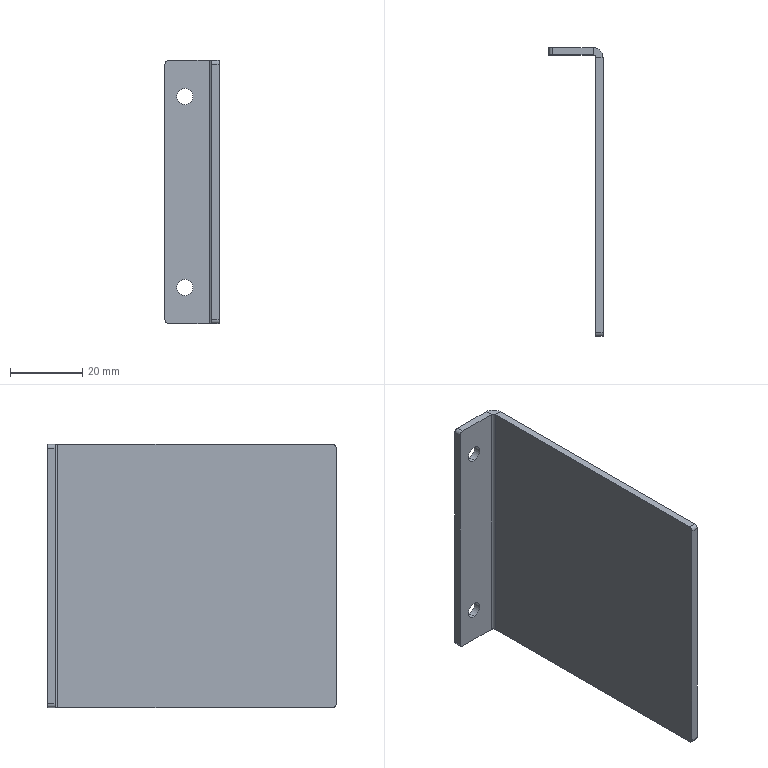Part | STEP file | 11-FG-B07311 | 1 solid | 22 faces | box 15 x 80 x 73 mm | volume 13404 mm3 | plane 12 | cylinder 10 | commonest cylinder face diameters 2 x4 4.5 x4 1.473 x1 5.473 x1
STEP:
#1=CARTESIAN_POINT('',(5.5,-2.,7.75));
#2=VERTEX_POINT('',#1);
#3=CARTESIAN_POINT('',(5.5,-2.,12.25));
#4=VERTEX_POINT('',#3);
#5=CARTESIAN_POINT('',(5.5,-2.,10.));
#6=DIRECTION('',(0.,1.,0.));
#7=DIRECTION('',(0.,0.,1.));
#8=AXIS2_PLACEMENT_3D('',#5,#6,#7);
#9=CIRCLE('',#8,2.25);
#10=EDGE_CURVE('',#2,#4,#9,.T.);
#11=ORIENTED_EDGE('',*,*,#10,.F.);
#12=CARTESIAN_POINT('',(5.5,0.,7.75));
#13=VERTEX_POINT('',#12);
#14=CARTESIAN_POINT('',(5.5,-10.,7.75));
#15=DIRECTION('',(0.,1.,0.));
#16=VECTOR('',#15,1000.);
#17=LINE('',#14,#16);
#18=EDGE_CURVE('',#2,#13,#17,.T.);
#19=ORIENTED_EDGE('',*,*,#18,.T.);
#20=CARTESIAN_POINT('',(5.5,0.,12.25));
#21=VERTEX_POINT('',#20);
#22=CARTESIAN_POINT('',(5.5,0.,10.));
#23=DIRECTION('',(0.,1.,0.));
#24=DIRECTION('',(0.,0.,1.));
#25=AXIS2_PLACEMENT_3D('',#22,#23,#24);
#26=CIRCLE('',#25,2.25);
#27=EDGE_CURVE('',#13,#21,#26,.T.);
#28=ORIENTED_EDGE('',*,*,#27,.T.);
#29=CARTESIAN_POINT('',(5.5,-10.,12.25));
#30=DIRECTION('',(0.,1.,0.));
#31=VECTOR('',#30,1000.);
#32=LINE('',#29,#31);
#33=EDGE_CURVE('',#4,#21,#32,.T.);
#34=ORIENTED_EDGE('',*,*,#33,.F.);
#35=EDGE_LOOP('',(#11,#19,#28,#34));
#36=FACE_OUTER_BOUND('',#35,.T.);
#37=CARTESIAN_POINT('',(5.5,-10.,10.));
#38=DIRECTION('',(0.,1.,0.));
#39=DIRECTION('',(0.,0.,1.));
#40=AXIS2_PLACEMENT_3D('',#37,#38,#39);
#41=CYLINDRICAL_SURFACE('',#40,2.25);
#42=ADVANCED_FACE('',(#36),#41,.F.);
#43=CARTESIAN_POINT('',(5.5,-2.,60.75));
#44=VERTEX_POINT('',#43);
#45=CARTESIAN_POINT('',(5.5,-2.,65.25));
#46=VERTEX_POINT('',#45);
#47=CARTESIAN_POINT('',(5.5,-2.,63.));
#48=DIRECTION('',(0.,1.,0.));
#49=DIRECTION('',(0.,0.,1.));
#50=AXIS2_PLACEMENT_3D('',#47,#48,#49);
#51=CIRCLE('',#50,2.25);
#52=EDGE_CURVE('',#44,#46,#51,.T.);
#53=ORIENTED_EDGE('',*,*,#52,.F.);
#54=CARTESIAN_POINT('',(5.5,0.,60.75));
#55=VERTEX_POINT('',#54);
#56=CARTESIAN_POINT('',(5.5,-10.,60.75));
#57=DIRECTION('',(0.,1.,0.));
#58=VECTOR('',#57,1000.);
#59=LINE('',#56,#58);
#60=EDGE_CURVE('',#44,#55,#59,.T.);
#61=ORIENTED_EDGE('',*,*,#60,.T.);
#62=CARTESIAN_POINT('',(5.5,0.,65.25));
#63=VERTEX_POINT('',#62);
#64=CARTESIAN_POINT('',(5.5,0.,63.));
#65=DIRECTION('',(0.,1.,0.));
#66=DIRECTION('',(0.,0.,1.));
#67=AXIS2_PLACEMENT_3D('',#64,#65,#66);
#68=CIRCLE('',#67,2.25);
#69=EDGE_CURVE('',#55,#63,#68,.T.);
#70=ORIENTED_EDGE('',*,*,#69,.T.);
#71=CARTESIAN_POINT('',(5.5,-10.,65.25));
#72=DIRECTION('',(0.,1.,0.));
#73=VECTOR('',#72,1000.);
#74=LINE('',#71,#73);
#75=EDGE_CURVE('',#46,#63,#74,.T.);
#76=ORIENTED_EDGE('',*,*,#75,.F.);
#77=EDGE_LOOP('',(#53,#61,#70,#76));
#78=FACE_OUTER_BOUND('',#77,.T.);
#79=CARTESIAN_POINT('',(5.5,-10.,63.));
#80=DIRECTION('',(0.,1.,0.));
#81=DIRECTION('',(0.,0.,1.));
#82=AXIS2_PLACEMENT_3D('',#79,#80,#81);
#83=CYLINDRICAL_SURFACE('',#82,2.25);
#84=ADVANCED_FACE('',(#78),#83,.F.);
#85=CARTESIAN_POINT('',(15.,-2.737,73.));
#86=VERTEX_POINT('',#85);
#87=CARTESIAN_POINT('',(13.,-2.737,73.));
#88=VERTEX_POINT('',#87);
#89=CARTESIAN_POINT('',(15.,-2.737,73.));
#90=DIRECTION('',(-1.,0.,0.));
#91=VECTOR('',#90,1000.);
#92=LINE('',#89,#91);
#93=EDGE_CURVE('',#86,#88,#92,.T.);
#94=ORIENTED_EDGE('',*,*,#93,.F.);
#95=CARTESIAN_POINT('',(12.263,0.,73.));
#96=VERTEX_POINT('',#95);
#97=CARTESIAN_POINT('',(12.263,-2.737,73.));
#98=DIRECTION('',(0.,0.,-1.));
#99=DIRECTION('',(1.,0.,0.));
#100=AXIS2_PLACEMENT_3D('',#97,#98,#99);
#101=CIRCLE('',#100,2.737);
#102=EDGE_CURVE('',#96,#86,#101,.T.);
#103=ORIENTED_EDGE('',*,*,#102,.F.);
#104=CARTESIAN_POINT('',(12.263,-2.,73.));
#105=VERTEX_POINT('',#104);
#106=CARTESIAN_POINT('',(12.263,-2.,73.));
#107=DIRECTION('',(0.,1.,0.));
#108=VECTOR('',#107,1000.);
#109=LINE('',#106,#108);
#110=EDGE_CURVE('',#105,#96,#109,.T.);
#111=ORIENTED_EDGE('',*,*,#110,.F.);
#112=CARTESIAN_POINT('',(12.263,-2.737,73.));
#113=DIRECTION('',(0.,0.,-1.));
#114=DIRECTION('',(1.,0.,0.));
#115=AXIS2_PLACEMENT_3D('',#112,#113,#114);
#116=CIRCLE('',#115,0.7366);
#117=EDGE_CURVE('',#105,#88,#116,.T.);
#118=ORIENTED_EDGE('',*,*,#117,.T.);
#119=EDGE_LOOP('',(#94,#103,#111,#118));
#120=FACE_OUTER_BOUND('',#119,.T.);
#121=CARTESIAN_POINT('',(15.,-2.737,73.));
#122=DIRECTION('',(0.,0.,1.));
#123=DIRECTION('',(1.,0.,0.));
#124=AXIS2_PLACEMENT_3D('',#121,#122,#123);
#125=PLANE('',#124);
#126=ADVANCED_FACE('',(#120),#125,.T.);
#127=CARTESIAN_POINT('',(13.,-79.,73.));
#128=VERTEX_POINT('',#127);
#129=CARTESIAN_POINT('',(13.,0.,73.));
#130=DIRECTION('',(0.,-1.,0.));
#131=VECTOR('',#130,1000.);
#132=LINE('',#129,#131);
#133=EDGE_CURVE('',#88,#128,#132,.T.);
#134=ORIENTED_EDGE('',*,*,#133,.T.);
#135=CARTESIAN_POINT('',(15.,-79.,73.));
#136=VERTEX_POINT('',#135);
#137=CARTESIAN_POINT('',(12.263,-79.,73.));
#138=DIRECTION('',(1.,0.,0.));
#139=VECTOR('',#138,1000.);
#140=LINE('',#137,#139);
#141=EDGE_CURVE('',#128,#136,#140,.T.);
#142=ORIENTED_EDGE('',*,*,#141,.T.);
#143=CARTESIAN_POINT('',(15.,0.,73.));
#144=DIRECTION('',(0.,-1.,0.));
#145=VECTOR('',#144,1000.);
#146=LINE('',#143,#145);
#147=EDGE_CURVE('',#86,#136,#146,.T.);
#148=ORIENTED_EDGE('',*,*,#147,.F.);
#149=ORIENTED_EDGE('',*,*,#93,.T.);
#150=EDGE_LOOP('',(#134,#142,#148,#149));
#151=FACE_OUTER_BOUND('',#150,.T.);
#152=CARTESIAN_POINT('',(12.263,-2.,73.));
#153=DIRECTION('',(0.,0.,1.));
#154=DIRECTION('',(1.,0.,0.));
#155=AXIS2_PLACEMENT_3D('',#152,#153,#154);
#156=PLANE('',#155);
#157=ADVANCED_FACE('',(#151),#156,.T.);
#158=CARTESIAN_POINT('',(12.263,0.,0.));
#159=VERTEX_POINT('',#158);
#160=CARTESIAN_POINT('',(12.263,-2.,0.));
#161=VERTEX_POINT('',#160);
#162=CARTESIAN_POINT('',(12.263,0.,0.));
#163=DIRECTION('',(0.,-1.,0.));
#164=VECTOR('',#163,1000.);
#165=LINE('',#162,#164);
#166=EDGE_CURVE('',#159,#161,#165,.T.);
#167=ORIENTED_EDGE('',*,*,#166,.F.);
#168=CARTESIAN_POINT('',(15.,-2.737,0.));
#169=VERTEX_POINT('',#168);
#170=CARTESIAN_POINT('',(12.263,-2.737,0.));
#171=DIRECTION('',(0.,0.,-1.));
#172=DIRECTION('',(1.,0.,0.));
#173=AXIS2_PLACEMENT_3D('',#170,#171,#172);
#174=CIRCLE('',#173,2.737);
#175=EDGE_CURVE('',#159,#169,#174,.T.);
#176=ORIENTED_EDGE('',*,*,#175,.T.);
#177=CARTESIAN_POINT('',(13.,-2.737,0.));
#178=VERTEX_POINT('',#177);
#179=CARTESIAN_POINT('',(13.,-2.737,0.));
#180=DIRECTION('',(1.,0.,0.));
#181=VECTOR('',#180,1000.);
#182=LINE('',#179,#181);
#183=EDGE_CURVE('',#178,#169,#182,.T.);
#184=ORIENTED_EDGE('',*,*,#183,.F.);
#185=CARTESIAN_POINT('',(12.263,-2.737,0.));
#186=DIRECTION('',(0.,0.,-1.));
#187=DIRECTION('',(1.,0.,0.));
#188=AXIS2_PLACEMENT_3D('',#185,#186,#187);
#189=CIRCLE('',#188,0.7366);
#190=EDGE_CURVE('',#161,#178,#189,.T.);
#191=ORIENTED_EDGE('',*,*,#190,.F.);
#192=EDGE_LOOP('',(#167,#176,#184,#191));
#193=FACE_OUTER_BOUND('',#192,.T.);
#194=CARTESIAN_POINT('',(12.263,0.,0.));
#195=DIRECTION('',(0.,0.,-1.));
#196=DIRECTION('',(-1.,0.,0.));
#197=AXIS2_PLACEMENT_3D('',#194,#195,#196);
#198=PLANE('',#197);
#199=ADVANCED_FACE('',(#193),#198,.T.);
#200=CARTESIAN_POINT('',(1.,-2.,0.));
#201=VERTEX_POINT('',#200);
#202=CARTESIAN_POINT('',(0.,-2.,0.));
#203=DIRECTION('',(1.,0.,0.));
#204=VECTOR('',#203,1000.);
#205=LINE('',#202,#204);
#206=EDGE_CURVE('',#201,#161,#205,.T.);
#207=ORIENTED_EDGE('',*,*,#206,.F.);
#208=CARTESIAN_POINT('',(1.,0.,0.));
#209=VERTEX_POINT('',#208);
#210=CARTESIAN_POINT('',(1.,-2.737,0.));
#211=DIRECTION('',(0.,1.,0.));
#212=VECTOR('',#211,1000.);
#213=LINE('',#210,#212);
#214=EDGE_CURVE('',#201,#209,#213,.T.);
#215=ORIENTED_EDGE('',*,*,#214,.T.);
#216=CARTESIAN_POINT('',(0.,0.,0.));
#217=DIRECTION('',(1.,0.,0.));
#218=VECTOR('',#217,1000.);
#219=LINE('',#216,#218);
#220=EDGE_CURVE('',#209,#159,#219,.T.);
#221=ORIENTED_EDGE('',*,*,#220,.T.);
#222=ORIENTED_EDGE('',*,*,#166,.T.);
#223=EDGE_LOOP('',(#207,#215,#221,#222));
#224=FACE_OUTER_BOUND('',#223,.T.);
#225=CARTESIAN_POINT('',(13.,-2.737,0.));
#226=DIRECTION('',(0.,0.,-1.));
#227=DIRECTION('',(-1.,0.,0.));
#228=AXIS2_PLACEMENT_3D('',#225,#226,#227);
#229=PLANE('',#228);
#230=ADVANCED_FACE('',(#224),#229,.T.);
#231=CARTESIAN_POINT('',(13.,-80.,72.));
#232=VERTEX_POINT('',#231);
#233=CARTESIAN_POINT('',(13.,-80.,1.));
#234=VERTEX_POINT('',#233);
#235=CARTESIAN_POINT('',(13.,-80.,73.));
#236=DIRECTION('',(0.,0.,-1.));
#237=VECTOR('',#236,1000.);
#238=LINE('',#235,#237);
#239=EDGE_CURVE('',#232,#234,#238,.T.);
#240=ORIENTED_EDGE('',*,*,#239,.F.);
#241=CARTESIAN_POINT('',(13.,-79.,72.));
#242=DIRECTION('',(-1.,0.,0.));
#243=DIRECTION('',(0.,1.,0.));
#244=AXIS2_PLACEMENT_3D('',#241,#242,#243);
#245=CIRCLE('',#244,1.);
#246=EDGE_CURVE('',#232,#128,#245,.T.);
#247=ORIENTED_EDGE('',*,*,#246,.T.);
#248=ORIENTED_EDGE('',*,*,#133,.F.);
#249=CARTESIAN_POINT('',(13.,-2.737,73.));
#250=DIRECTION('',(0.,0.,-1.));
#251=VECTOR('',#250,1000.);
#252=LINE('',#249,#251);
#253=EDGE_CURVE('',#88,#178,#252,.T.);
#254=ORIENTED_EDGE('',*,*,#253,.T.);
#255=CARTESIAN_POINT('',(13.,-79.,0.));
#256=VERTEX_POINT('',#255);
#257=CARTESIAN_POINT('',(13.,0.,0.));
#258=DIRECTION('',(0.,-1.,0.));
#259=VECTOR('',#258,1000.);
#260=LINE('',#257,#259);
#261=EDGE_CURVE('',#178,#256,#260,.T.);
#262=ORIENTED_EDGE('',*,*,#261,.T.);
#263=CARTESIAN_POINT('',(13.,-79.,1.));
#264=DIRECTION('',(-1.,0.,0.));
#265=DIRECTION('',(0.,1.,0.));
#266=AXIS2_PLACEMENT_3D('',#263,#264,#265);
#267=CIRCLE('',#266,1.);
#268=EDGE_CURVE('',#256,#234,#267,.T.);
#269=ORIENTED_EDGE('',*,*,#268,.T.);
#270=EDGE_LOOP('',(#240,#247,#248,#254,#262,#269));
#271=FACE_OUTER_BOUND('',#270,.T.);
#272=CARTESIAN_POINT('',(13.,0.,73.));
#273=DIRECTION('',(1.,0.,0.));
#274=DIRECTION('',(0.,1.,0.));
#275=AXIS2_PLACEMENT_3D('',#272,#273,#274);
#276=PLANE('',#275);
#277=ADVANCED_FACE('',(#271),#276,.F.);
#278=CARTESIAN_POINT('',(15.,-80.,72.));
#279=VERTEX_POINT('',#278);
#280=CARTESIAN_POINT('',(15.,-80.,1.));
#281=VERTEX_POINT('',#280);
#282=CARTESIAN_POINT('',(15.,-80.,73.));
#283=DIRECTION('',(0.,0.,-1.));
#284=VECTOR('',#283,1000.);
#285=LINE('',#282,#284);
#286=EDGE_CURVE('',#279,#281,#285,.T.);
#287=ORIENTED_EDGE('',*,*,#286,.F.);
#288=CARTESIAN_POINT('',(15.,-80.,72.));
#289=DIRECTION('',(-1.,0.,0.));
#290=VECTOR('',#289,1000.);
#291=LINE('',#288,#290);
#292=EDGE_CURVE('',#279,#232,#291,.T.);
#293=ORIENTED_EDGE('',*,*,#292,.T.);
#294=ORIENTED_EDGE('',*,*,#239,.T.);
#295=CARTESIAN_POINT('',(15.,-80.,1.));
#296=DIRECTION('',(1.,0.,0.));
#297=VECTOR('',#296,1000.);
#298=LINE('',#295,#297);
#299=EDGE_CURVE('',#234,#281,#298,.T.);
#300=ORIENTED_EDGE('',*,*,#299,.T.);
#301=EDGE_LOOP('',(#287,#293,#294,#300));
#302=FACE_OUTER_BOUND('',#301,.T.);
#303=CARTESIAN_POINT('',(15.,-80.,73.));
#304=DIRECTION('',(0.,-1.,0.));
#305=DIRECTION('',(0.,0.,-1.));
#306=AXIS2_PLACEMENT_3D('',#303,#304,#305);
#307=PLANE('',#306);
#308=ADVANCED_FACE('',(#302),#307,.T.);
#309=ORIENTED_EDGE('',*,*,#147,.T.);
#310=CARTESIAN_POINT('',(15.,-79.,72.));
#311=DIRECTION('',(1.,0.,0.));
#312=DIRECTION('',(0.,1.,0.));
#313=AXIS2_PLACEMENT_3D('',#310,#311,#312);
#314=CIRCLE('',#313,1.);
#315=EDGE_CURVE('',#136,#279,#314,.T.);
#316=ORIENTED_EDGE('',*,*,#315,.T.);
#317=ORIENTED_EDGE('',*,*,#286,.T.);
#318=CARTESIAN_POINT('',(15.,-79.,0.));
#319=VERTEX_POINT('',#318);
#320=CARTESIAN_POINT('',(15.,-79.,1.));
#321=DIRECTION('',(1.,0.,0.));
#322=DIRECTION('',(0.,1.,0.));
#323=AXIS2_PLACEMENT_3D('',#320,#321,#322);
#324=CIRCLE('',#323,1.);
#325=EDGE_CURVE('',#281,#319,#324,.T.);
#326=ORIENTED_EDGE('',*,*,#325,.T.);
#327=CARTESIAN_POINT('',(15.,0.,0.));
#328=DIRECTION('',(0.,-1.,0.));
#329=VECTOR('',#328,1000.);
#330=LINE('',#327,#329);
#331=EDGE_CURVE('',#169,#319,#330,.T.);
#332=ORIENTED_EDGE('',*,*,#331,.F.);
#333=CARTESIAN_POINT('',(15.,-2.737,73.));
#334=DIRECTION('',(0.,0.,-1.));
#335=VECTOR('',#334,1000.);
#336=LINE('',#333,#335);
#337=EDGE_CURVE('',#86,#169,#336,.T.);
#338=ORIENTED_EDGE('',*,*,#337,.F.);
#339=EDGE_LOOP('',(#309,#316,#317,#326,#332,#338));
#340=FACE_OUTER_BOUND('',#339,.T.);
#341=CARTESIAN_POINT('',(15.,0.,73.));
#342=DIRECTION('',(1.,0.,0.));
#343=DIRECTION('',(0.,1.,0.));
#344=AXIS2_PLACEMENT_3D('',#341,#342,#343);
#345=PLANE('',#344);
#346=ADVANCED_FACE('',(#340),#345,.T.);
#347=ORIENTED_EDGE('',*,*,#175,.F.);
#348=CARTESIAN_POINT('',(12.263,0.,73.));
#349=DIRECTION('',(0.,0.,-1.));
#350=VECTOR('',#349,1000.);
#351=LINE('',#348,#350);
#352=EDGE_CURVE('',#96,#159,#351,.T.);
#353=ORIENTED_EDGE('',*,*,#352,.F.);
#354=ORIENTED_EDGE('',*,*,#102,.T.);
#355=ORIENTED_EDGE('',*,*,#337,.T.);
#356=EDGE_LOOP('',(#347,#353,#354,#355));
#357=FACE_OUTER_BOUND('',#356,.T.);
#358=CARTESIAN_POINT('',(12.263,-2.737,73.));
#359=DIRECTION('',(0.,0.,-1.));
#360=DIRECTION('',(-1.,0.,0.));
#361=AXIS2_PLACEMENT_3D('',#358,#359,#360);
#362=CYLINDRICAL_SURFACE('',#361,2.737);
#363=ADVANCED_FACE('',(#357),#362,.T.);
#364=CARTESIAN_POINT('',(5.5,0.,10.));
#365=DIRECTION('',(0.,1.,0.));
#366=DIRECTION('',(0.,0.,1.));
#367=AXIS2_PLACEMENT_3D('',#364,#365,#366);
#368=CIRCLE('',#367,2.25);
#369=EDGE_CURVE('',#21,#13,#368,.T.);
#370=ORIENTED_EDGE('',*,*,#369,.F.);
#371=ORIENTED_EDGE('',*,*,#27,.F.);
#372=EDGE_LOOP('',(#370,#371));
#373=FACE_BOUND('',#372,.T.);
#374=CARTESIAN_POINT('',(5.5,0.,63.));
#375=DIRECTION('',(0.,1.,0.));
#376=DIRECTION('',(0.,0.,1.));
#377=AXIS2_PLACEMENT_3D('',#374,#375,#376);
#378=CIRCLE('',#377,2.25);
#379=EDGE_CURVE('',#63,#55,#378,.T.);
#380=ORIENTED_EDGE('',*,*,#379,.F.);
#381=ORIENTED_EDGE('',*,*,#69,.F.);
#382=EDGE_LOOP('',(#380,#381));
#383=FACE_BOUND('',#382,.T.);
#384=ORIENTED_EDGE('',*,*,#220,.F.);
#385=CARTESIAN_POINT('',(0.,0.,1.));
#386=VERTEX_POINT('',#385);
#387=CARTESIAN_POINT('',(1.,0.,1.));
#388=DIRECTION('',(0.,1.,0.));
#389=DIRECTION('',(0.,0.,1.));
#390=AXIS2_PLACEMENT_3D('',#387,#388,#389);
#391=CIRCLE('',#390,1.);
#392=EDGE_CURVE('',#209,#386,#391,.T.);
#393=ORIENTED_EDGE('',*,*,#392,.T.);
#394=CARTESIAN_POINT('',(0.,0.,72.));
#395=VERTEX_POINT('',#394);
#396=CARTESIAN_POINT('',(0.,0.,73.));
#397=DIRECTION('',(0.,0.,-1.));
#398=VECTOR('',#397,1000.);
#399=LINE('',#396,#398);
#400=EDGE_CURVE('',#395,#386,#399,.T.);
#401=ORIENTED_EDGE('',*,*,#400,.F.);
#402=CARTESIAN_POINT('',(1.,0.,73.));
#403=VERTEX_POINT('',#402);
#404=CARTESIAN_POINT('',(1.,0.,72.));
#405=DIRECTION('',(0.,1.,0.));
#406=DIRECTION('',(0.,0.,1.));
#407=AXIS2_PLACEMENT_3D('',#404,#405,#406);
#408=CIRCLE('',#407,1.);
#409=EDGE_CURVE('',#395,#403,#408,.T.);
#410=ORIENTED_EDGE('',*,*,#409,.T.);
#411=CARTESIAN_POINT('',(0.,0.,73.));
#412=DIRECTION('',(1.,0.,0.));
#413=VECTOR('',#412,1000.);
#414=LINE('',#411,#413);
#415=EDGE_CURVE('',#403,#96,#414,.T.);
#416=ORIENTED_EDGE('',*,*,#415,.T.);
#417=ORIENTED_EDGE('',*,*,#352,.T.);
#418=EDGE_LOOP('',(#384,#393,#401,#410,#416,#417));
#419=FACE_OUTER_BOUND('',#418,.T.);
#420=CARTESIAN_POINT('',(0.,0.,73.));
#421=DIRECTION('',(0.,1.,0.));
#422=DIRECTION('',(0.,0.,1.));
#423=AXIS2_PLACEMENT_3D('',#420,#421,#422);
#424=PLANE('',#423);
#425=ADVANCED_FACE('',(#373,#383,#419),#424,.T.);
#426=ORIENTED_EDGE('',*,*,#400,.T.);
#427=CARTESIAN_POINT('',(0.,-2.,1.));
#428=VERTEX_POINT('',#427);
#429=CARTESIAN_POINT('',(0.,-2.,1.));
#430=DIRECTION('',(0.,-1.,0.));
#431=VECTOR('',#430,1000.);
#432=LINE('',#429,#431);
#433=EDGE_CURVE('',#386,#428,#432,.T.);
#434=ORIENTED_EDGE('',*,*,#433,.T.);
#435=CARTESIAN_POINT('',(0.,-2.,72.));
#436=VERTEX_POINT('',#435);
#437=CARTESIAN_POINT('',(0.,-2.,73.));
#438=DIRECTION('',(0.,0.,-1.));
#439=VECTOR('',#438,1000.);
#440=LINE('',#437,#439);
#441=EDGE_CURVE('',#436,#428,#440,.T.);
#442=ORIENTED_EDGE('',*,*,#441,.F.);
#443=CARTESIAN_POINT('',(0.,-2.,72.));
#444=DIRECTION('',(0.,1.,0.));
#445=VECTOR('',#444,1000.);
#446=LINE('',#443,#445);
#447=EDGE_CURVE('',#436,#395,#446,.T.);
#448=ORIENTED_EDGE('',*,*,#447,.T.);
#449=EDGE_LOOP('',(#426,#434,#442,#448));
#450=FACE_OUTER_BOUND('',#449,.T.);
#451=CARTESIAN_POINT('',(0.,-2.,73.));
#452=DIRECTION('',(-1.,0.,0.));
#453=DIRECTION('',(0.,0.,1.));
#454=AXIS2_PLACEMENT_3D('',#451,#452,#453);
#455=PLANE('',#454);
#456=ADVANCED_FACE('',(#450),#455,.T.);
#457=CARTESIAN_POINT('',(5.5,-2.,10.));
#458=DIRECTION('',(0.,1.,0.));
#459=DIRECTION('',(0.,0.,1.));
#460=AXIS2_PLACEMENT_3D('',#457,#458,#459);
#461=CIRCLE('',#460,2.25);
#462=EDGE_CURVE('',#4,#2,#461,.T.);
#463=ORIENTED_EDGE('',*,*,#462,.T.);
#464=ORIENTED_EDGE('',*,*,#10,.T.);
#465=EDGE_LOOP('',(#463,#464));
#466=FACE_BOUND('',#465,.T.);
#467=CARTESIAN_POINT('',(5.5,-2.,63.));
#468=DIRECTION('',(0.,1.,0.));
#469=DIRECTION('',(0.,0.,1.));
#470=AXIS2_PLACEMENT_3D('',#467,#468,#469);
#471=CIRCLE('',#470,2.25);
#472=EDGE_CURVE('',#46,#44,#471,.T.);
#473=ORIENTED_EDGE('',*,*,#472,.T.);
#474=ORIENTED_EDGE('',*,*,#52,.T.);
#475=EDGE_LOOP('',(#473,#474));
#476=FACE_BOUND('',#475,.T.);
#477=ORIENTED_EDGE('',*,*,#441,.T.);
#478=CARTESIAN_POINT('',(1.,-2.,1.));
#479=DIRECTION('',(0.,-1.,0.));
#480=DIRECTION('',(0.,0.,1.));
#481=AXIS2_PLACEMENT_3D('',#478,#479,#480);
#482=CIRCLE('',#481,1.);
#483=EDGE_CURVE('',#428,#201,#482,.T.);
#484=ORIENTED_EDGE('',*,*,#483,.T.);
#485=ORIENTED_EDGE('',*,*,#206,.T.);
#486=CARTESIAN_POINT('',(12.263,-2.,73.));
#487=DIRECTION('',(0.,0.,-1.));
#488=VECTOR('',#487,1000.);
#489=LINE('',#486,#488);
#490=EDGE_CURVE('',#105,#161,#489,.T.);
#491=ORIENTED_EDGE('',*,*,#490,.F.);
#492=CARTESIAN_POINT('',(1.,-2.,73.));
#493=VERTEX_POINT('',#492);
#494=CARTESIAN_POINT('',(0.,-2.,73.));
#495=DIRECTION('',(1.,0.,0.));
#496=VECTOR('',#495,1000.);
#497=LINE('',#494,#496);
#498=EDGE_CURVE('',#493,#105,#497,.T.);
#499=ORIENTED_EDGE('',*,*,#498,.F.);
#500=CARTESIAN_POINT('',(1.,-2.,72.));
#501=DIRECTION('',(0.,-1.,0.));
#502=DIRECTION('',(0.,0.,1.));
#503=AXIS2_PLACEMENT_3D('',#500,#501,#502);
#504=CIRCLE('',#503,1.);
#505=EDGE_CURVE('',#493,#436,#504,.T.);
#506=ORIENTED_EDGE('',*,*,#505,.T.);
#507=EDGE_LOOP('',(#477,#484,#485,#491,#499,#506));
#508=FACE_OUTER_BOUND('',#507,.T.);
#509=CARTESIAN_POINT('',(0.,-2.,73.));
#510=DIRECTION('',(0.,1.,0.));
#511=DIRECTION('',(0.,0.,1.));
#512=AXIS2_PLACEMENT_3D('',#509,#510,#511);
#513=PLANE('',#512);
#514=ADVANCED_FACE('',(#466,#476,#508),#513,.F.);
#515=ORIENTED_EDGE('',*,*,#190,.T.);
#516=ORIENTED_EDGE('',*,*,#253,.F.);
#517=ORIENTED_EDGE('',*,*,#117,.F.);
#518=ORIENTED_EDGE('',*,*,#490,.T.);
#519=EDGE_LOOP('',(#515,#516,#517,#518));
#520=FACE_OUTER_BOUND('',#519,.T.);
#521=CARTESIAN_POINT('',(12.263,-2.737,73.));
#522=DIRECTION('',(0.,0.,-1.));
#523=DIRECTION('',(-1.,0.,0.));
#524=AXIS2_PLACEMENT_3D('',#521,#522,#523);
#525=CYLINDRICAL_SURFACE('',#524,0.7366);
#526=ADVANCED_FACE('',(#520),#525,.F.);
#527=ORIENTED_EDGE('',*,*,#415,.F.);
#528=CARTESIAN_POINT('',(1.,-2.737,73.));
#529=DIRECTION('',(0.,-1.,0.));
#530=VECTOR('',#529,1000.);
#531=LINE('',#528,#530);
#532=EDGE_CURVE('',#403,#493,#531,.T.);
#533=ORIENTED_EDGE('',*,*,#532,.T.);
#534=ORIENTED_EDGE('',*,*,#498,.T.);
#535=ORIENTED_EDGE('',*,*,#110,.T.);
#536=EDGE_LOOP('',(#527,#533,#534,#535));
#537=FACE_OUTER_BOUND('',#536,.T.);
#538=CARTESIAN_POINT('',(12.263,-2.737,73.));
#539=DIRECTION('',(0.,0.,1.));
#540=DIRECTION('',(1.,0.,0.));
#541=AXIS2_PLACEMENT_3D('',#538,#539,#540);
#542=PLANE('',#541);
#543=ADVANCED_FACE('',(#537),#542,.T.);
#544=ORIENTED_EDGE('',*,*,#331,.T.);
#545=CARTESIAN_POINT('',(13.,-79.,0.));
#546=DIRECTION('',(-1.,0.,0.));
#547=VECTOR('',#546,1000.);
#548=LINE('',#545,#547);
#549=EDGE_CURVE('',#319,#256,#548,.T.);
#550=ORIENTED_EDGE('',*,*,#549,.T.);
#551=ORIENTED_EDGE('',*,*,#261,.F.);
#552=ORIENTED_EDGE('',*,*,#183,.T.);
#553=EDGE_LOOP('',(#544,#550,#551,#552));
#554=FACE_OUTER_BOUND('',#553,.T.);
#555=CARTESIAN_POINT('',(12.263,-2.737,0.));
#556=DIRECTION('',(0.,0.,1.));
#557=DIRECTION('',(1.,0.,0.));
#558=AXIS2_PLACEMENT_3D('',#555,#556,#557);
#559=PLANE('',#558);
#560=ADVANCED_FACE('',(#554),#559,.F.);
#561=ORIENTED_EDGE('',*,*,#315,.F.);
#562=ORIENTED_EDGE('',*,*,#141,.F.);
#563=ORIENTED_EDGE('',*,*,#246,.F.);
#564=ORIENTED_EDGE('',*,*,#292,.F.);
#565=EDGE_LOOP('',(#561,#562,#563,#564));
#566=FACE_OUTER_BOUND('',#565,.T.);
#567=CARTESIAN_POINT('',(15.,-79.,72.));
#568=DIRECTION('',(-1.,0.,0.));
#569=DIRECTION('',(0.,0.,1.));
#570=AXIS2_PLACEMENT_3D('',#567,#568,#569);
#571=CYLINDRICAL_SURFACE('',#570,1.);
#572=ADVANCED_FACE('',(#566),#571,.T.);
#573=ORIENTED_EDGE('',*,*,#325,.F.);
#574=ORIENTED_EDGE('',*,*,#299,.F.);
#575=ORIENTED_EDGE('',*,*,#268,.F.);
#576=ORIENTED_EDGE('',*,*,#549,.F.);
#577=EDGE_LOOP('',(#573,#574,#575,#576));
#578=FACE_OUTER_BOUND('',#577,.T.);
#579=CARTESIAN_POINT('',(12.263,-79.,1.));
#580=DIRECTION('',(1.,0.,0.));
#581=DIRECTION('',(0.,0.,-1.));
#582=AXIS2_PLACEMENT_3D('',#579,#580,#581);
#583=CYLINDRICAL_SURFACE('',#582,1.);
#584=ADVANCED_FACE('',(#578),#583,.T.);
#585=ORIENTED_EDGE('',*,*,#483,.F.);
#586=ORIENTED_EDGE('',*,*,#433,.F.);
#587=ORIENTED_EDGE('',*,*,#392,.F.);
#588=ORIENTED_EDGE('',*,*,#214,.F.);
#589=EDGE_LOOP('',(#585,#586,#587,#588));
#590=FACE_OUTER_BOUND('',#589,.T.);
#591=CARTESIAN_POINT('',(1.,-2.737,1.));
#592=DIRECTION('',(0.,1.,0.));
#593=DIRECTION('',(0.,0.,1.));
#594=AXIS2_PLACEMENT_3D('',#591,#592,#593);
#595=CYLINDRICAL_SURFACE('',#594,1.);
#596=ADVANCED_FACE('',(#590),#595,.T.);
#597=ORIENTED_EDGE('',*,*,#505,.F.);
#598=ORIENTED_EDGE('',*,*,#532,.F.);
#599=ORIENTED_EDGE('',*,*,#409,.F.);
#600=ORIENTED_EDGE('',*,*,#447,.F.);
#601=EDGE_LOOP('',(#597,#598,#599,#600));
#602=FACE_OUTER_BOUND('',#601,.T.);
#603=CARTESIAN_POINT('',(1.,-2.,72.));
#604=DIRECTION('',(0.,1.,0.));
#605=DIRECTION('',(0.,0.,1.));
#606=AXIS2_PLACEMENT_3D('',#603,#604,#605);
#607=CYLINDRICAL_SURFACE('',#606,1.);
#608=ADVANCED_FACE('',(#602),#607,.T.);
#609=ORIENTED_EDGE('',*,*,#60,.F.);
#610=ORIENTED_EDGE('',*,*,#472,.F.);
#611=ORIENTED_EDGE('',*,*,#75,.T.);
#612=ORIENTED_EDGE('',*,*,#379,.T.);
#613=EDGE_LOOP('',(#609,#610,#611,#612));
#614=FACE_OUTER_BOUND('',#613,.T.);
#615=CARTESIAN_POINT('',(5.5,-10.,63.));
#616=DIRECTION('',(0.,1.,0.));
#617=DIRECTION('',(0.,0.,1.));
#618=AXIS2_PLACEMENT_3D('',#615,#616,#617);
#619=CYLINDRICAL_SURFACE('',#618,2.25);
#620=ADVANCED_FACE('',(#614),#619,.F.);
#621=ORIENTED_EDGE('',*,*,#18,.F.);
#622=ORIENTED_EDGE('',*,*,#462,.F.);
#623=ORIENTED_EDGE('',*,*,#33,.T.);
#624=ORIENTED_EDGE('',*,*,#369,.T.);
#625=EDGE_LOOP('',(#621,#622,#623,#624));
#626=FACE_OUTER_BOUND('',#625,.T.);
#627=CARTESIAN_POINT('',(5.5,-10.,10.));
#628=DIRECTION('',(0.,1.,0.));
#629=DIRECTION('',(0.,0.,1.));
#630=AXIS2_PLACEMENT_3D('',#627,#628,#629);
#631=CYLINDRICAL_SURFACE('',#630,2.25);
#632=ADVANCED_FACE('',(#626),#631,.F.);
#633=CLOSED_SHELL('',(#42,#84,#126,#157,#199,#230,#277,#308,#346,#363,#425,#456,#514,#526,#543,#560,#572,#584,#596,#608,#620,#632));
#634=MANIFOLD_SOLID_BREP('',#633);
#635=CARTESIAN_POINT('',(0.,0.,0.));
#636=DIRECTION('',(0.,0.,1.));
#637=DIRECTION('',(1.,0.,0.));
#638=AXIS2_PLACEMENT_3D('',#635,#636,#637);
#639=(LENGTH_UNIT()NAMED_UNIT(*)SI_UNIT(.MILLI.,.METRE.));
#640=UNCERTAINTY_MEASURE_WITH_UNIT(LENGTH_MEASURE(0.00001),#639,'','');
#641=(NAMED_UNIT(*)PLANE_ANGLE_UNIT()SI_UNIT($,.RADIAN.));
#642=(NAMED_UNIT(*)SI_UNIT($,.STERADIAN.)SOLID_ANGLE_UNIT());
#643=(GEOMETRIC_REPRESENTATION_CONTEXT(3)GLOBAL_UNCERTAINTY_ASSIGNED_CONTEXT((#640))GLOBAL_UNIT_ASSIGNED_CONTEXT((#639,#641,#642))REPRESENTATION_CONTEXT('',''));
#644=ADVANCED_BREP_SHAPE_REPRESENTATION('',(#634,#638),#643);